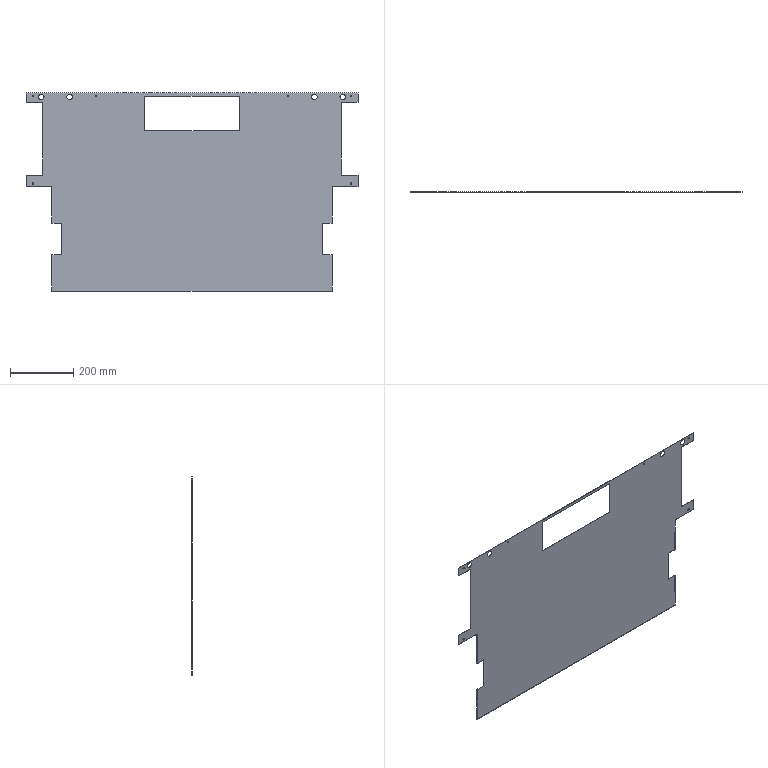Part | 1 solid | 50 faces | box 1050 x 1 x 626.5 mm | volume 539189 mm3 | plane 30 | cylinder 20 | commonest cylinder face diameters 5 x12 18 x8